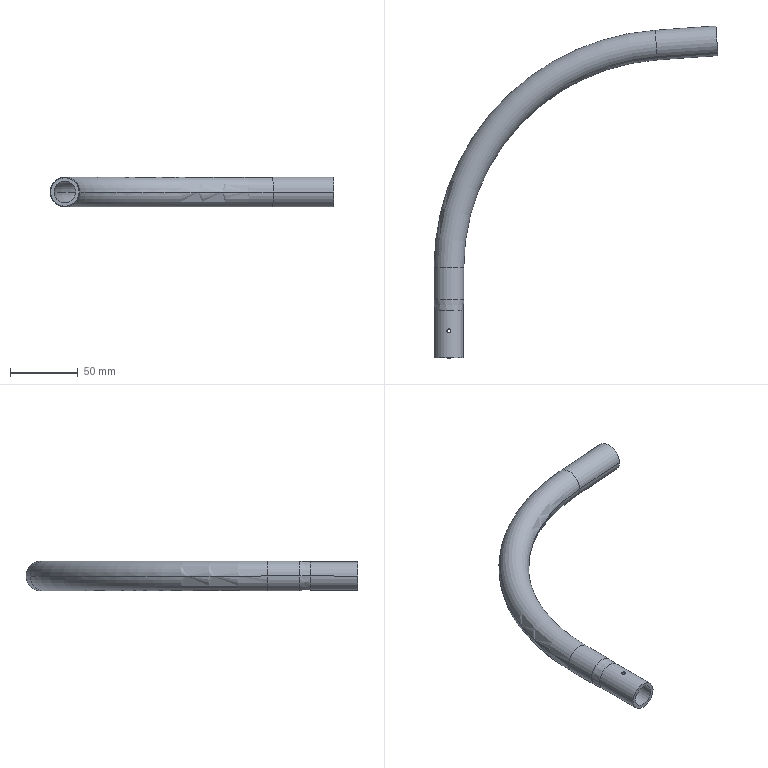Part | STEP file | 31E-01158WG10 | 1 solid | 22 faces | box 210.148 x 245.71 x 22 mm | volume 63051 mm3 | cylinder 14 | torus 4 | cone 2 | plane 2 | commonest cylinder face diameters 3 x4 16 x4 22 x4 21 x2
STEP:
#1=CARTESIAN_POINT('',(-1.316,20.719,-10.417));
#2=VERTEX_POINT('',#1);
#3=CARTESIAN_POINT('',(-1.316,20.719,-7.891));
#4=VERTEX_POINT('',#3);
#5=CARTESIAN_POINT('',(-1.316,20.719,-3.345));
#6=DIRECTION('',(0.,0.,-1.));
#7=VECTOR('',#6,1.);
#8=LINE('',#5,#7);
#9=EDGE_CURVE('',#2,#4,#8,.F.);
#10=ORIENTED_EDGE('',*,*,#9,.F.);
#11=CARTESIAN_POINT('',(1.316,19.281,-10.417));
#12=VERTEX_POINT('',#11);
#13=CARTESIAN_POINT('',(-1.316,20.719,-10.417));
#14=CARTESIAN_POINT('',(-1.132,21.056,-10.44));
#15=CARTESIAN_POINT('',(-0.8411,21.333,-10.473));
#16=CARTESIAN_POINT('',(-0.4667,21.506,-10.502));
#17=CARTESIAN_POINT('',(0.1367,21.567,-10.509));
#18=CARTESIAN_POINT('',(0.6816,21.357,-10.48));
#19=CARTESIAN_POINT('',(0.8505,21.258,-10.467));
#20=CARTESIAN_POINT('',(1.286,20.898,-10.426));
#21=CARTESIAN_POINT('',(1.526,20.366,-10.389));
#22=CARTESIAN_POINT('',(1.57,19.977,-10.381));
#23=CARTESIAN_POINT('',(1.492,19.602,-10.395));
#24=CARTESIAN_POINT('',(1.316,19.281,-10.417));
#25=B_SPLINE_CURVE_WITH_KNOTS('',5,(#13,#14,#15,#16,#17,#18,#19,#20,#21,#22,#23,#24),.UNSPECIFIED.,.F.,.U.,(6,3,3,6),(0.,2.718,4.081,6.673),.UNSPECIFIED.);
#26=EDGE_CURVE('',#2,#12,#25,.T.);
#27=ORIENTED_EDGE('',*,*,#26,.T.);
#28=CARTESIAN_POINT('',(1.316,19.281,-7.891));
#29=VERTEX_POINT('',#28);
#30=CARTESIAN_POINT('',(1.316,19.281,-3.345));
#31=DIRECTION('',(0.,0.,-1.));
#32=VECTOR('',#31,1.);
#33=LINE('',#30,#32);
#34=EDGE_CURVE('',#12,#29,#33,.F.);
#35=ORIENTED_EDGE('',*,*,#34,.T.);
#36=CARTESIAN_POINT('',(1.316,19.281,-7.891));
#37=CARTESIAN_POINT('',(1.5,19.618,-7.86));
#38=CARTESIAN_POINT('',(1.577,20.014,-7.842));
#39=CARTESIAN_POINT('',(1.518,20.425,-7.856));
#40=CARTESIAN_POINT('',(1.244,20.963,-7.911));
#41=CARTESIAN_POINT('',(0.7734,21.307,-7.965));
#42=CARTESIAN_POINT('',(0.5986,21.396,-7.981));
#43=CARTESIAN_POINT('',(0.05895,21.567,-8.012));
#44=CARTESIAN_POINT('',(-0.5205,21.481,-7.997));
#45=CARTESIAN_POINT('',(-0.8688,21.306,-7.961));
#46=CARTESIAN_POINT('',(-1.141,21.04,-7.92));
#47=CARTESIAN_POINT('',(-1.316,20.719,-7.891));
#48=B_SPLINE_CURVE_WITH_KNOTS('',5,(#36,#37,#38,#39,#40,#41,#42,#43,#44,#45,#46,#47),.UNSPECIFIED.,.F.,.U.,(6,3,3,6),(0.,2.721,4.087,6.679),.UNSPECIFIED.);
#49=EDGE_CURVE('',#29,#4,#48,.T.);
#50=ORIENTED_EDGE('',*,*,#49,.T.);
#51=EDGE_LOOP('',(#10,#27,#35,#50));
#52=FACE_OUTER_BOUND('',#51,.T.);
#53=CARTESIAN_POINT('',(0.,20.,-0.1));
#54=DIRECTION('',(0.,0.,-1.));
#55=DIRECTION('',(0.8776,-0.4794,0.));
#56=AXIS2_PLACEMENT_3D('',#53,#54,#55);
#57=CYLINDRICAL_SURFACE('',#56,1.5);
#58=ADVANCED_FACE('',(#52),#57,.F.);
#59=CARTESIAN_POINT('',(-8.,0.,0.));
#60=VERTEX_POINT('',#59);
#61=CARTESIAN_POINT('',(-8.,67.,0.));
#62=VERTEX_POINT('',#61);
#63=CARTESIAN_POINT('',(-8.,33.5,0.));
#64=DIRECTION('',(0.,1.,0.));
#65=VECTOR('',#64,1.);
#66=LINE('',#63,#65);
#67=EDGE_CURVE('',#60,#62,#66,.T.);
#68=ORIENTED_EDGE('',*,*,#67,.F.);
#69=CARTESIAN_POINT('',(8.,0.,0.));
#70=VERTEX_POINT('',#69);
#71=CARTESIAN_POINT('',(0.,0.,0.));
#72=DIRECTION('',(0.,1.,0.));
#73=AXIS2_PLACEMENT_3D('',#71,#72,$);
#74=CIRCLE('',#73,8.);
#75=EDGE_CURVE('',#70,#60,#74,.T.);
#76=ORIENTED_EDGE('',*,*,#75,.F.);
#77=CARTESIAN_POINT('',(8.,67.,0.));
#78=VERTEX_POINT('',#77);
#79=CARTESIAN_POINT('',(8.,33.5,0.));
#80=DIRECTION('',(0.,1.,0.));
#81=VECTOR('',#80,1.);
#82=LINE('',#79,#81);
#83=EDGE_CURVE('',#70,#78,#82,.T.);
#84=ORIENTED_EDGE('',*,*,#83,.T.);
#85=CARTESIAN_POINT('',(0.,67.,0.));
#86=DIRECTION('',(0.,1.,0.));
#87=AXIS2_PLACEMENT_3D('',#85,#86,$);
#88=CIRCLE('',#87,8.);
#89=EDGE_CURVE('',#62,#78,#88,.F.);
#90=ORIENTED_EDGE('',*,*,#89,.F.);
#91=EDGE_LOOP('',(#68,#76,#84,#90));
#92=FACE_OUTER_BOUND('',#91,.T.);
#93=ORIENTED_EDGE('',*,*,#49,.F.);
#94=CARTESIAN_POINT('',(1.316,19.281,-7.891));
#95=CARTESIAN_POINT('',(1.132,18.944,-7.922));
#96=CARTESIAN_POINT('',(0.8414,18.667,-7.965));
#97=CARTESIAN_POINT('',(0.4674,18.493,-8.002));
#98=CARTESIAN_POINT('',(-0.137,18.433,-8.012));
#99=CARTESIAN_POINT('',(-0.682,18.643,-7.974));
#100=CARTESIAN_POINT('',(-0.8508,18.742,-7.957));
#101=CARTESIAN_POINT('',(-1.285,19.102,-7.903));
#102=CARTESIAN_POINT('',(-1.526,19.633,-7.854));
#103=CARTESIAN_POINT('',(-1.57,20.023,-7.844));
#104=CARTESIAN_POINT('',(-1.492,20.398,-7.862));
#105=CARTESIAN_POINT('',(-1.316,20.719,-7.891));
#106=B_SPLINE_CURVE_WITH_KNOTS('',5,(#94,#95,#96,#97,#98,#99,#100,#101,#102,#103,#104,#105),.UNSPECIFIED.,.F.,.U.,(6,3,3,6),(0.,2.721,4.086,6.679),.UNSPECIFIED.);
#107=EDGE_CURVE('',#29,#4,#106,.T.);
#108=ORIENTED_EDGE('',*,*,#107,.T.);
#109=EDGE_LOOP('',(#93,#108));
#110=FACE_BOUND('',#109,.T.);
#111=CARTESIAN_POINT('',(0.,33.5,0.));
#112=DIRECTION('',(0.,1.,0.));
#113=DIRECTION('',(1.,0.,0.));
#114=AXIS2_PLACEMENT_3D('',#111,#112,#113);
#115=CYLINDRICAL_SURFACE('',#114,8.);
#116=ADVANCED_FACE('',(#92,#110),#115,.F.);
#117=CARTESIAN_POINT('',(1.316,19.281,-10.417));
#118=CARTESIAN_POINT('',(1.132,18.944,-10.44));
#119=CARTESIAN_POINT('',(0.8411,18.667,-10.473));
#120=CARTESIAN_POINT('',(0.4667,18.494,-10.502));
#121=CARTESIAN_POINT('',(-0.1367,18.433,-10.509));
#122=CARTESIAN_POINT('',(-0.6816,18.643,-10.48));
#123=CARTESIAN_POINT('',(-0.8505,18.742,-10.467));
#124=CARTESIAN_POINT('',(-1.286,19.102,-10.426));
#125=CARTESIAN_POINT('',(-1.526,19.634,-10.389));
#126=CARTESIAN_POINT('',(-1.57,20.023,-10.381));
#127=CARTESIAN_POINT('',(-1.492,20.398,-10.395));
#128=CARTESIAN_POINT('',(-1.316,20.719,-10.417));
#129=B_SPLINE_CURVE_WITH_KNOTS('',5,(#117,#118,#119,#120,#121,#122,#123,#124,#125,#126,#127,#128),.UNSPECIFIED.,.F.,.U.,(6,3,3,6),(0.,2.718,4.081,6.673),.UNSPECIFIED.);
#130=EDGE_CURVE('',#12,#2,#129,.T.);
#131=ORIENTED_EDGE('',*,*,#130,.T.);
#132=ORIENTED_EDGE('',*,*,#9,.T.);
#133=ORIENTED_EDGE('',*,*,#107,.F.);
#134=ORIENTED_EDGE('',*,*,#34,.F.);
#135=EDGE_LOOP('',(#131,#132,#133,#134));
#136=FACE_OUTER_BOUND('',#135,.T.);
#137=ADVANCED_FACE('',(#136),#57,.F.);
#138=CARTESIAN_POINT('',(-10.5,35.,0.));
#139=VERTEX_POINT('',#138);
#140=CARTESIAN_POINT('',(10.5,35.,0.));
#141=VERTEX_POINT('',#140);
#142=CARTESIAN_POINT('',(0.,35.,0.));
#143=DIRECTION('',(0.,-1.,0.));
#144=AXIS2_PLACEMENT_3D('',#142,#143,$);
#145=CIRCLE('',#144,10.5);
#146=EDGE_CURVE('',#139,#141,#145,.T.);
#147=ORIENTED_EDGE('',*,*,#146,.T.);
#148=CARTESIAN_POINT('',(10.5,0.,0.));
#149=VERTEX_POINT('',#148);
#150=CARTESIAN_POINT('',(10.5,17.5,0.));
#151=DIRECTION('',(0.,-1.,0.));
#152=VECTOR('',#151,1.);
#153=LINE('',#150,#152);
#154=EDGE_CURVE('',#149,#141,#153,.F.);
#155=ORIENTED_EDGE('',*,*,#154,.F.);
#156=CARTESIAN_POINT('',(-10.5,0.,0.));
#157=VERTEX_POINT('',#156);
#158=CARTESIAN_POINT('',(0.,0.,0.));
#159=DIRECTION('',(0.,-1.,0.));
#160=AXIS2_PLACEMENT_3D('',#158,#159,$);
#161=CIRCLE('',#160,10.5);
#162=EDGE_CURVE('',#157,#149,#161,.T.);
#163=ORIENTED_EDGE('',*,*,#162,.F.);
#164=CARTESIAN_POINT('',(-10.5,17.5,0.));
#165=DIRECTION('',(0.,-1.,0.));
#166=VECTOR('',#165,1.);
#167=LINE('',#164,#166);
#168=EDGE_CURVE('',#157,#139,#167,.F.);
#169=ORIENTED_EDGE('',*,*,#168,.T.);
#170=EDGE_LOOP('',(#147,#155,#163,#169));
#171=FACE_OUTER_BOUND('',#170,.T.);
#172=ORIENTED_EDGE('',*,*,#130,.F.);
#173=ORIENTED_EDGE('',*,*,#26,.F.);
#174=EDGE_LOOP('',(#172,#173));
#175=FACE_BOUND('',#174,.T.);
#176=CARTESIAN_POINT('',(0.,17.5,0.));
#177=DIRECTION('',(0.,-1.,0.));
#178=DIRECTION('',(1.,0.,0.));
#179=AXIS2_PLACEMENT_3D('',#176,#177,#178);
#180=CYLINDRICAL_SURFACE('',#179,10.5);
#181=ADVANCED_FACE('',(#171,#175),#180,.T.);
#182=ORIENTED_EDGE('',*,*,#83,.F.);
#183=CARTESIAN_POINT('',(0.,0.,0.));
#184=DIRECTION('',(0.,1.,0.));
#185=AXIS2_PLACEMENT_3D('',#183,#184,$);
#186=CIRCLE('',#185,8.);
#187=EDGE_CURVE('',#60,#70,#186,.T.);
#188=ORIENTED_EDGE('',*,*,#187,.F.);
#189=ORIENTED_EDGE('',*,*,#67,.T.);
#190=CARTESIAN_POINT('',(0.,67.,0.));
#191=DIRECTION('',(0.,1.,0.));
#192=AXIS2_PLACEMENT_3D('',#190,#191,$);
#193=CIRCLE('',#192,8.);
#194=EDGE_CURVE('',#78,#62,#193,.F.);
#195=ORIENTED_EDGE('',*,*,#194,.F.);
#196=EDGE_LOOP('',(#182,#188,#189,#195));
#197=FACE_OUTER_BOUND('',#196,.T.);
#198=CARTESIAN_POINT('',(1.316,20.719,7.891));
#199=VERTEX_POINT('',#198);
#200=CARTESIAN_POINT('',(-1.316,19.281,7.891));
#201=VERTEX_POINT('',#200);
#202=CARTESIAN_POINT('',(1.316,20.719,7.891));
#203=CARTESIAN_POINT('',(1.5,20.382,7.86));
#204=CARTESIAN_POINT('',(1.577,19.986,7.842));
#205=CARTESIAN_POINT('',(1.518,19.575,7.856));
#206=CARTESIAN_POINT('',(1.244,19.037,7.911));
#207=CARTESIAN_POINT('',(0.7734,18.693,7.965));
#208=CARTESIAN_POINT('',(0.5986,18.604,7.981));
#209=CARTESIAN_POINT('',(0.05895,18.433,8.012));
#210=CARTESIAN_POINT('',(-0.5205,18.519,7.997));
#211=CARTESIAN_POINT('',(-0.8688,18.694,7.961));
#212=CARTESIAN_POINT('',(-1.141,18.96,7.92));
#213=CARTESIAN_POINT('',(-1.316,19.281,7.891));
#214=B_SPLINE_CURVE_WITH_KNOTS('',5,(#202,#203,#204,#205,#206,#207,#208,#209,#210,#211,#212,#213),.UNSPECIFIED.,.F.,.U.,(6,3,3,6),(0.,2.721,4.087,6.679),.UNSPECIFIED.);
#215=EDGE_CURVE('',#199,#201,#214,.T.);
#216=ORIENTED_EDGE('',*,*,#215,.F.);
#217=CARTESIAN_POINT('',(-1.316,20.719,7.891));
#218=VERTEX_POINT('',#217);
#219=CARTESIAN_POINT('',(1.316,20.719,7.891));
#220=CARTESIAN_POINT('',(1.132,21.056,7.922));
#221=CARTESIAN_POINT('',(0.8414,21.333,7.965));
#222=CARTESIAN_POINT('',(0.4674,21.507,8.002));
#223=CARTESIAN_POINT('',(-0.2065,21.574,8.013));
#224=CARTESIAN_POINT('',(-0.8064,21.305,7.965));
#225=CARTESIAN_POINT('',(-1.02,21.146,7.938));
#226=CARTESIAN_POINT('',(-1.192,20.946,7.912));
#227=CARTESIAN_POINT('',(-1.316,20.719,7.891));
#228=B_SPLINE_CURVE_WITH_KNOTS('',5,(#219,#220,#221,#222,#223,#224,#225,#226,#227),.UNSPECIFIED.,.F.,.U.,(6,3,6),(0.,2.721,4.555),.UNSPECIFIED.);
#229=EDGE_CURVE('',#199,#218,#228,.T.);
#230=ORIENTED_EDGE('',*,*,#229,.T.);
#231=CARTESIAN_POINT('',(-1.316,20.719,7.891));
#232=CARTESIAN_POINT('',(-1.496,20.391,7.861));
#233=CARTESIAN_POINT('',(-1.567,20.,7.843));
#234=CARTESIAN_POINT('',(-1.496,19.609,7.861));
#235=CARTESIAN_POINT('',(-1.316,19.281,7.891));
#236=B_SPLINE_CURVE_WITH_KNOTS('',4,(#231,#232,#233,#234,#235),.UNSPECIFIED.,.F.,.U.,(5,5),(4.555,6.679),.UNSPECIFIED.);
#237=EDGE_CURVE('',#218,#201,#236,.T.);
#238=ORIENTED_EDGE('',*,*,#237,.T.);
#239=EDGE_LOOP('',(#216,#230,#238));
#240=FACE_BOUND('',#239,.T.);
#241=CARTESIAN_POINT('',(0.,33.5,0.));
#242=DIRECTION('',(0.,1.,0.));
#243=DIRECTION('',(-1.,0.,0.));
#244=AXIS2_PLACEMENT_3D('',#241,#242,#243);
#245=CYLINDRICAL_SURFACE('',#244,8.);
#246=ADVANCED_FACE('',(#197,#240),#245,.F.);
#247=CARTESIAN_POINT('',(0.,35.,0.));
#248=DIRECTION('',(0.,-1.,0.));
#249=AXIS2_PLACEMENT_3D('',#247,#248,$);
#250=CIRCLE('',#249,10.5);
#251=EDGE_CURVE('',#141,#139,#250,.T.);
#252=ORIENTED_EDGE('',*,*,#251,.T.);
#253=ORIENTED_EDGE('',*,*,#168,.F.);
#254=CARTESIAN_POINT('',(0.,0.,0.));
#255=DIRECTION('',(0.,-1.,0.));
#256=AXIS2_PLACEMENT_3D('',#254,#255,$);
#257=CIRCLE('',#256,10.5);
#258=EDGE_CURVE('',#149,#157,#257,.T.);
#259=ORIENTED_EDGE('',*,*,#258,.F.);
#260=ORIENTED_EDGE('',*,*,#154,.T.);
#261=EDGE_LOOP('',(#252,#253,#259,#260));
#262=FACE_OUTER_BOUND('',#261,.T.);
#263=CARTESIAN_POINT('',(-1.316,20.719,10.417));
#264=VERTEX_POINT('',#263);
#265=CARTESIAN_POINT('',(-1.316,19.281,10.417));
#266=VERTEX_POINT('',#265);
#267=CARTESIAN_POINT('',(-1.316,20.719,10.417));
#268=CARTESIAN_POINT('',(-1.496,20.39,10.394));
#269=CARTESIAN_POINT('',(-1.567,20.,10.381));
#270=CARTESIAN_POINT('',(-1.496,19.61,10.394));
#271=CARTESIAN_POINT('',(-1.316,19.281,10.417));
#272=B_SPLINE_CURVE_WITH_KNOTS('',4,(#267,#268,#269,#270,#271),.UNSPECIFIED.,.F.,.U.,(5,5),(4.55,6.673),.UNSPECIFIED.);
#273=EDGE_CURVE('',#264,#266,#272,.T.);
#274=ORIENTED_EDGE('',*,*,#273,.F.);
#275=CARTESIAN_POINT('',(1.316,20.719,10.417));
#276=VERTEX_POINT('',#275);
#277=CARTESIAN_POINT('',(1.316,20.719,10.417));
#278=CARTESIAN_POINT('',(1.008,21.283,10.456));
#279=CARTESIAN_POINT('',(0.4018,21.686,10.529));
#280=CARTESIAN_POINT('',(-0.4018,21.686,10.529));
#281=CARTESIAN_POINT('',(-1.008,21.283,10.456));
#282=CARTESIAN_POINT('',(-1.316,20.719,10.417));
#283=B_SPLINE_CURVE_WITH_KNOTS('',5,(#277,#278,#279,#280,#281,#282),.UNSPECIFIED.,.F.,.U.,(6,6),(0.,4.55),.UNSPECIFIED.);
#284=EDGE_CURVE('',#276,#264,#283,.T.);
#285=ORIENTED_EDGE('',*,*,#284,.F.);
#286=CARTESIAN_POINT('',(-1.316,19.281,10.417));
#287=CARTESIAN_POINT('',(-1.132,18.944,10.44));
#288=CARTESIAN_POINT('',(-0.8411,18.667,10.473));
#289=CARTESIAN_POINT('',(-0.4667,18.494,10.502));
#290=CARTESIAN_POINT('',(0.1367,18.433,10.509));
#291=CARTESIAN_POINT('',(0.6816,18.643,10.48));
#292=CARTESIAN_POINT('',(0.8505,18.742,10.467));
#293=CARTESIAN_POINT('',(1.286,19.102,10.426));
#294=CARTESIAN_POINT('',(1.526,19.634,10.389));
#295=CARTESIAN_POINT('',(1.57,20.023,10.381));
#296=CARTESIAN_POINT('',(1.492,20.398,10.395));
#297=CARTESIAN_POINT('',(1.316,20.719,10.417));
#298=B_SPLINE_CURVE_WITH_KNOTS('',5,(#286,#287,#288,#289,#290,#291,#292,#293,#294,#295,#296,#297),.UNSPECIFIED.,.F.,.U.,(6,3,3,6),(0.,2.718,4.081,6.673),.UNSPECIFIED.);
#299=EDGE_CURVE('',#266,#276,#298,.T.);
#300=ORIENTED_EDGE('',*,*,#299,.F.);
#301=EDGE_LOOP('',(#274,#285,#300));
#302=FACE_BOUND('',#301,.T.);
#303=ADVANCED_FACE('',(#262,#302),#180,.T.);
#304=CARTESIAN_POINT('',(-11.,43.,0.));
#305=VERTEX_POINT('',#304);
#306=CARTESIAN_POINT('',(-10.75,39.,0.));
#307=DIRECTION('',(-0.06238,0.9981,0.));
#308=VECTOR('',#307,1.);
#309=LINE('',#306,#308);
#310=EDGE_CURVE('',#139,#305,#309,.T.);
#311=ORIENTED_EDGE('',*,*,#310,.T.);
#312=CARTESIAN_POINT('',(11.,43.,0.));
#313=VERTEX_POINT('',#312);
#314=CARTESIAN_POINT('',(0.,43.,0.));
#315=DIRECTION('',(0.,-1.,0.));
#316=AXIS2_PLACEMENT_3D('',#314,#315,$);
#317=CIRCLE('',#316,11.);
#318=EDGE_CURVE('',#305,#313,#317,.T.);
#319=ORIENTED_EDGE('',*,*,#318,.T.);
#320=CARTESIAN_POINT('',(10.75,39.,0.));
#321=DIRECTION('',(0.06238,0.9981,0.));
#322=VECTOR('',#321,1.);
#323=LINE('',#320,#322);
#324=EDGE_CURVE('',#141,#313,#323,.T.);
#325=ORIENTED_EDGE('',*,*,#324,.F.);
#326=ORIENTED_EDGE('',*,*,#146,.F.);
#327=EDGE_LOOP('',(#311,#319,#325,#326));
#328=FACE_OUTER_BOUND('',#327,.T.);
#329=CARTESIAN_POINT('',(0.,-133.,0.));
#330=DIRECTION('',(0.,1.,0.));
#331=DIRECTION('',(-0.9072,0.,0.4207));
#332=AXIS2_PLACEMENT_3D('',#329,#330,#331);
#333=CONICAL_SURFACE('',#332,0.,0.06242);
#334=ADVANCED_FACE('',(#328),#333,.T.);
#335=CARTESIAN_POINT('',(-1.316,20.719,3.345));
#336=DIRECTION('',(0.,0.,1.));
#337=VECTOR('',#336,1.);
#338=LINE('',#335,#337);
#339=EDGE_CURVE('',#218,#264,#338,.T.);
#340=ORIENTED_EDGE('',*,*,#339,.F.);
#341=ORIENTED_EDGE('',*,*,#229,.F.);
#342=CARTESIAN_POINT('',(1.316,20.719,3.345));
#343=DIRECTION('',(0.,0.,1.));
#344=VECTOR('',#343,1.);
#345=LINE('',#342,#344);
#346=EDGE_CURVE('',#199,#276,#345,.T.);
#347=ORIENTED_EDGE('',*,*,#346,.T.);
#348=ORIENTED_EDGE('',*,*,#284,.T.);
#349=EDGE_LOOP('',(#340,#341,#347,#348));
#350=FACE_OUTER_BOUND('',#349,.T.);
#351=CARTESIAN_POINT('',(0.,20.,0.1));
#352=DIRECTION('',(0.,0.,1.));
#353=DIRECTION('',(0.8776,0.4794,0.));
#354=AXIS2_PLACEMENT_3D('',#351,#352,#353);
#355=CYLINDRICAL_SURFACE('',#354,1.5);
#356=ADVANCED_FACE('',(#350),#355,.F.);
#357=ORIENTED_EDGE('',*,*,#324,.T.);
#358=CARTESIAN_POINT('',(0.,43.,0.));
#359=DIRECTION('',(0.,-1.,0.));
#360=AXIS2_PLACEMENT_3D('',#358,#359,$);
#361=CIRCLE('',#360,11.);
#362=EDGE_CURVE('',#313,#305,#361,.T.);
#363=ORIENTED_EDGE('',*,*,#362,.T.);
#364=ORIENTED_EDGE('',*,*,#310,.F.);
#365=ORIENTED_EDGE('',*,*,#251,.F.);
#366=EDGE_LOOP('',(#357,#363,#364,#365));
#367=FACE_OUTER_BOUND('',#366,.T.);
#368=CARTESIAN_POINT('',(0.,-133.,0.));
#369=DIRECTION('',(0.,1.,0.));
#370=DIRECTION('',(0.9092,0.,-0.4163));
#371=AXIS2_PLACEMENT_3D('',#368,#369,#370);
#372=CONICAL_SURFACE('',#371,0.,0.06242);
#373=ADVANCED_FACE('',(#367),#372,.T.);
#374=CARTESIAN_POINT('',(-11.,67.,0.));
#375=VERTEX_POINT('',#374);
#376=CARTESIAN_POINT('',(-11.,33.5,0.));
#377=DIRECTION('',(0.,1.,0.));
#378=VECTOR('',#377,1.);
#379=LINE('',#376,#378);
#380=EDGE_CURVE('',#305,#375,#379,.T.);
#381=ORIENTED_EDGE('',*,*,#380,.T.);
#382=CARTESIAN_POINT('',(11.,67.,0.));
#383=VERTEX_POINT('',#382);
#384=CARTESIAN_POINT('',(0.,67.,0.));
#385=DIRECTION('',(0.,1.,0.));
#386=AXIS2_PLACEMENT_3D('',#384,#385,$);
#387=CIRCLE('',#386,11.);
#388=EDGE_CURVE('',#375,#383,#387,.F.);
#389=ORIENTED_EDGE('',*,*,#388,.T.);
#390=CARTESIAN_POINT('',(11.,33.5,0.));
#391=DIRECTION('',(0.,1.,0.));
#392=VECTOR('',#391,1.);
#393=LINE('',#390,#392);
#394=EDGE_CURVE('',#313,#383,#393,.T.);
#395=ORIENTED_EDGE('',*,*,#394,.F.);
#396=ORIENTED_EDGE('',*,*,#318,.F.);
#397=EDGE_LOOP('',(#381,#389,#395,#396));
#398=FACE_OUTER_BOUND('',#397,.T.);
#399=CARTESIAN_POINT('',(0.,33.5,0.));
#400=DIRECTION('',(0.,1.,0.));
#401=DIRECTION('',(1.,0.,0.));
#402=AXIS2_PLACEMENT_3D('',#399,#400,#401);
#403=CYLINDRICAL_SURFACE('',#402,11.);
#404=ADVANCED_FACE('',(#398),#403,.T.);
#405=ORIENTED_EDGE('',*,*,#394,.T.);
#406=CARTESIAN_POINT('',(0.,67.,0.));
#407=DIRECTION('',(0.,1.,0.));
#408=AXIS2_PLACEMENT_3D('',#406,#407,$);
#409=CIRCLE('',#408,11.);
#410=EDGE_CURVE('',#383,#375,#409,.F.);
#411=ORIENTED_EDGE('',*,*,#410,.T.);
#412=ORIENTED_EDGE('',*,*,#380,.F.);
#413=ORIENTED_EDGE('',*,*,#362,.F.);
#414=EDGE_LOOP('',(#405,#411,#412,#413));
#415=FACE_OUTER_BOUND('',#414,.T.);
#416=CARTESIAN_POINT('',(0.,33.5,0.));
#417=DIRECTION('',(0.,1.,0.));
#418=DIRECTION('',(-1.,0.,0.));
#419=AXIS2_PLACEMENT_3D('',#416,#417,#418);
#420=CYLINDRICAL_SURFACE('',#419,11.);
#421=ADVANCED_FACE('',(#415),#420,.T.);
#422=CARTESIAN_POINT('',(152.723,242.571,0.));
#423=VERTEX_POINT('',#422);
#424=CARTESIAN_POINT('',(165.,67.,0.));
#425=DIRECTION('',(0.,0.,1.));
#426=AXIS2_PLACEMENT_3D('',#424,#425,$);
#427=CIRCLE('',#426,176.);
#428=EDGE_CURVE('',#423,#375,#427,.T.);
#429=ORIENTED_EDGE('',*,*,#428,.F.);
#430=CARTESIAN_POINT('',(154.258,220.625,0.));
#431=VERTEX_POINT('',#430);
#432=CARTESIAN_POINT('',(153.49,231.598,0.));
#433=DIRECTION('',(0.9976,0.06976,0.));
#434=AXIS2_PLACEMENT_3D('',#432,#433,$);
#435=CIRCLE('',#434,11.);
#436=EDGE_CURVE('',#423,#431,#435,.F.);
#437=ORIENTED_EDGE('',*,*,#436,.T.);
#438=CARTESIAN_POINT('',(165.,67.,0.));
#439=DIRECTION('',(0.,0.,1.));
#440=AXIS2_PLACEMENT_3D('',#438,#439,$);
#441=CIRCLE('',#440,154.);
#442=EDGE_CURVE('',#431,#383,#441,.T.);
#443=ORIENTED_EDGE('',*,*,#442,.T.);
#444=ORIENTED_EDGE('',*,*,#388,.F.);
#445=EDGE_LOOP('',(#429,#437,#443,#444));
#446=FACE_OUTER_BOUND('',#445,.T.);
#447=CARTESIAN_POINT('',(165.,67.,0.));
#448=DIRECTION('',(0.,0.,1.));
#449=DIRECTION('',(-0.06976,0.9976,0.));
#450=AXIS2_PLACEMENT_3D('',#447,#448,#449);
#451=TOROIDAL_SURFACE('',#450,165.,11.);
#452=ADVANCED_FACE('',(#446),#451,.T.);
#453=ORIENTED_EDGE('',*,*,#442,.F.);
#454=CARTESIAN_POINT('',(153.49,231.598,0.));
#455=DIRECTION('',(0.9976,0.06976,0.));
#456=AXIS2_PLACEMENT_3D('',#454,#455,$);
#457=CIRCLE('',#456,11.);
#458=EDGE_CURVE('',#431,#423,#457,.F.);
#459=ORIENTED_EDGE('',*,*,#458,.T.);
#460=ORIENTED_EDGE('',*,*,#428,.T.);
#461=ORIENTED_EDGE('',*,*,#410,.F.);
#462=EDGE_LOOP('',(#453,#459,#460,#461));
#463=FACE_OUTER_BOUND('',#462,.T.);
#464=CARTESIAN_POINT('',(165.,67.,0.));
#465=DIRECTION('',(0.,0.,1.));
#466=DIRECTION('',(-0.06976,0.9976,0.));
#467=AXIS2_PLACEMENT_3D('',#464,#465,#466);
#468=TOROIDAL_SURFACE('',#467,165.,11.);
#469=ADVANCED_FACE('',(#463),#468,.T.);
#470=CARTESIAN_POINT('',(199.148,223.764,0.));
#471=VERTEX_POINT('',#470);
#472=CARTESIAN_POINT('',(197.613,245.71,0.));
#473=VERTEX_POINT('',#472);
#474=CARTESIAN_POINT('',(198.381,234.737,0.));
#475=DIRECTION('',(0.9976,0.06976,0.));
#476=AXIS2_PLACEMENT_3D('',#474,#475,$);
#477=CIRCLE('',#476,11.);
#478=EDGE_CURVE('',#471,#473,#477,.T.);
#479=ORIENTED_EDGE('',*,*,#478,.F.);
#480=CARTESIAN_POINT('',(176.703,222.194,0.));
#481=DIRECTION('',(0.9976,0.06976,0.));
#482=VECTOR('',#481,1.);
#483=LINE('',#480,#482);
#484=EDGE_CURVE('',#431,#471,#483,.T.);
#485=ORIENTED_EDGE('',*,*,#484,.F.);
#486=ORIENTED_EDGE('',*,*,#436,.F.);
#487=CARTESIAN_POINT('',(175.168,244.141,0.));
#488=DIRECTION('',(0.9976,0.06976,0.));
#489=VECTOR('',#488,1.);
#490=LINE('',#487,#489);
#491=EDGE_CURVE('',#423,#473,#490,.T.);
#492=ORIENTED_EDGE('',*,*,#491,.T.);
#493=EDGE_LOOP('',(#479,#485,#486,#492));
#494=FACE_OUTER_BOUND('',#493,.T.);
#495=CARTESIAN_POINT('',(175.935,233.168,0.));
#496=DIRECTION('',(0.9976,0.06976,0.));
#497=DIRECTION('',(0.06976,-0.9976,0.));
#498=AXIS2_PLACEMENT_3D('',#495,#496,#497);
#499=CYLINDRICAL_SURFACE('',#498,11.);
#500=ADVANCED_FACE('',(#494),#499,.T.);
#501=CARTESIAN_POINT('',(198.381,234.737,0.));
#502=DIRECTION('',(0.9976,0.06976,0.));
#503=AXIS2_PLACEMENT_3D('',#501,#502,$);
#504=CIRCLE('',#503,11.);
#505=EDGE_CURVE('',#473,#471,#504,.T.);
#506=ORIENTED_EDGE('',*,*,#505,.F.);
#507=ORIENTED_EDGE('',*,*,#491,.F.);
#508=ORIENTED_EDGE('',*,*,#458,.F.);
#509=ORIENTED_EDGE('',*,*,#484,.T.);
#510=EDGE_LOOP('',(#506,#507,#508,#509));
#511=FACE_OUTER_BOUND('',#510,.T.);
#512=CARTESIAN_POINT('',(175.935,233.168,0.));
#513=DIRECTION('',(0.9976,0.06976,0.));
#514=DIRECTION('',(-0.06976,0.9976,0.));
#515=AXIS2_PLACEMENT_3D('',#512,#513,#514);
#516=CYLINDRICAL_SURFACE('',#515,11.);
#517=ADVANCED_FACE('',(#511),#516,.T.);
#518=CARTESIAN_POINT('',(154.048,223.618,0.));
#519=VERTEX_POINT('',#518);
#520=CARTESIAN_POINT('',(198.939,226.757,0.));
#521=VERTEX_POINT('',#520);
#522=CARTESIAN_POINT('',(176.493,225.187,0.));
#523=DIRECTION('',(0.9976,0.06976,0.));
#524=VECTOR('',#523,1.);
#525=LINE('',#522,#524);
#526=EDGE_CURVE('',#519,#521,#525,.T.);
#527=ORIENTED_EDGE('',*,*,#526,.F.);
#528=CARTESIAN_POINT('',(152.932,239.579,0.));
#529=VERTEX_POINT('',#528);
#530=CARTESIAN_POINT('',(153.49,231.598,0.));
#531=DIRECTION('',(0.9976,0.06976,0.));
#532=AXIS2_PLACEMENT_3D('',#530,#531,$);
#533=CIRCLE('',#532,8.);
#534=EDGE_CURVE('',#519,#529,#533,.F.);
#535=ORIENTED_EDGE('',*,*,#534,.T.);
#536=CARTESIAN_POINT('',(197.823,242.718,0.));
#537=VERTEX_POINT('',#536);
#538=CARTESIAN_POINT('',(175.377,241.148,0.));
#539=DIRECTION('',(0.9976,0.06976,0.));
#540=VECTOR('',#539,1.);
#541=LINE('',#538,#540);
#542=EDGE_CURVE('',#529,#537,#541,.T.);
#543=ORIENTED_EDGE('',*,*,#542,.T.);
#544=CARTESIAN_POINT('',(198.381,234.737,0.));
#545=DIRECTION('',(0.9976,0.06976,0.));
#546=AXIS2_PLACEMENT_3D('',#544,#545,$);
#547=CIRCLE('',#546,8.);
#548=EDGE_CURVE('',#537,#521,#547,.T.);
#549=ORIENTED_EDGE('',*,*,#548,.T.);
#550=EDGE_LOOP('',(#527,#535,#543,#549));
#551=FACE_OUTER_BOUND('',#550,.T.);
#552=CARTESIAN_POINT('',(175.935,233.168,0.));
#553=DIRECTION('',(0.9976,0.06976,0.));
#554=DIRECTION('',(-0.06976,0.9976,0.));
#555=AXIS2_PLACEMENT_3D('',#552,#553,#554);
#556=CYLINDRICAL_SURFACE('',#555,8.);
#557=ADVANCED_FACE('',(#551),#556,.F.);
#558=ORIENTED_EDGE('',*,*,#542,.F.);
#559=CARTESIAN_POINT('',(153.49,231.598,0.));
#560=DIRECTION('',(0.9976,0.06976,0.));
#561=AXIS2_PLACEMENT_3D('',#559,#560,$);
#562=CIRCLE('',#561,8.);
#563=EDGE_CURVE('',#529,#519,#562,.F.);
#564=ORIENTED_EDGE('',*,*,#563,.T.);
#565=ORIENTED_EDGE('',*,*,#526,.T.);
#566=CARTESIAN_POINT('',(198.381,234.737,0.));
#567=DIRECTION('',(0.9976,0.06976,0.));
#568=AXIS2_PLACEMENT_3D('',#566,#567,$);
#569=CIRCLE('',#568,8.);
#570=EDGE_CURVE('',#521,#537,#569,.T.);
#571=ORIENTED_EDGE('',*,*,#570,.T.);
#572=EDGE_LOOP('',(#558,#564,#565,#571));
#573=FACE_OUTER_BOUND('',#572,.T.);
#574=CARTESIAN_POINT('',(175.935,233.168,0.));
#575=DIRECTION('',(0.9976,0.06976,0.));
#576=DIRECTION('',(0.06976,-0.9976,0.));
#577=AXIS2_PLACEMENT_3D('',#574,#575,#576);
#578=CYLINDRICAL_SURFACE('',#577,8.);
#579=ADVANCED_FACE('',(#573),#578,.F.);
#580=ORIENTED_EDGE('',*,*,#505,.T.);
#581=ORIENTED_EDGE('',*,*,#478,.T.);
#582=EDGE_LOOP('',(#580,#581));
#583=FACE_OUTER_BOUND('',#582,.T.);
#584=ORIENTED_EDGE('',*,*,#548,.F.);
#585=ORIENTED_EDGE('',*,*,#570,.F.);
#586=EDGE_LOOP('',(#584,#585));
#587=FACE_BOUND('',#586,.T.);
#588=CARTESIAN_POINT('',(198.381,234.737,0.));
#589=DIRECTION('',(0.9976,0.06976,0.));
#590=DIRECTION('',(-0.06976,0.9976,0.));
#591=AXIS2_PLACEMENT_3D('',#588,#589,#590);
#592=PLANE('',#591);
#593=ADVANCED_FACE('',(#583,#587),#592,.T.);
#594=ORIENTED_EDGE('',*,*,#194,.T.);
#595=CARTESIAN_POINT('',(165.,67.,0.));
#596=DIRECTION('',(0.,0.,1.));
#597=AXIS2_PLACEMENT_3D('',#595,#596,$);
#598=CIRCLE('',#597,173.);
#599=EDGE_CURVE('',#529,#62,#598,.T.);
#600=ORIENTED_EDGE('',*,*,#599,.F.);
#601=ORIENTED_EDGE('',*,*,#534,.F.);
#602=CARTESIAN_POINT('',(165.,67.,0.));
#603=DIRECTION('',(0.,0.,1.));
#604=AXIS2_PLACEMENT_3D('',#602,#603,$);
#605=CIRCLE('',#604,157.);
#606=EDGE_CURVE('',#519,#78,#605,.T.);
#607=ORIENTED_EDGE('',*,*,#606,.T.);
#608=EDGE_LOOP('',(#594,#600,#601,#607));
#609=FACE_OUTER_BOUND('',#608,.T.);
#610=CARTESIAN_POINT('',(165.,67.,0.));
#611=DIRECTION('',(0.,0.,1.));
#612=DIRECTION('',(-0.06976,0.9976,0.));
#613=AXIS2_PLACEMENT_3D('',#610,#611,#612);
#614=TOROIDAL_SURFACE('',#613,165.,8.);
#615=ADVANCED_FACE('',(#609),#614,.F.);
#616=ORIENTED_EDGE('',*,*,#162,.T.);
#617=ORIENTED_EDGE('',*,*,#258,.T.);
#618=EDGE_LOOP('',(#616,#617));
#619=FACE_OUTER_BOUND('',#618,.T.);
#620=ORIENTED_EDGE('',*,*,#187,.T.);
#621=ORIENTED_EDGE('',*,*,#75,.T.);
#622=EDGE_LOOP('',(#620,#621));
#623=FACE_BOUND('',#622,.T.);
#624=CARTESIAN_POINT('',(0.,0.,0.));
#625=DIRECTION('',(0.,1.,0.));
#626=DIRECTION('',(0.,0.,1.));
#627=AXIS2_PLACEMENT_3D('',#624,#625,#626);
#628=PLANE('',#627);
#629=ADVANCED_FACE('',(#619,#623),#628,.F.);
#630=ORIENTED_EDGE('',*,*,#89,.T.);
#631=ORIENTED_EDGE('',*,*,#606,.F.);
#632=ORIENTED_EDGE('',*,*,#563,.F.);
#633=ORIENTED_EDGE('',*,*,#599,.T.);
#634=EDGE_LOOP('',(#630,#631,#632,#633));
#635=FACE_OUTER_BOUND('',#634,.T.);
#636=CARTESIAN_POINT('',(165.,67.,0.));
#637=DIRECTION('',(0.,0.,1.));
#638=DIRECTION('',(-0.06976,0.9976,0.));
#639=AXIS2_PLACEMENT_3D('',#636,#637,#638);
#640=TOROIDAL_SURFACE('',#639,165.,8.);
#641=ADVANCED_FACE('',(#635),#640,.F.);
#642=ORIENTED_EDGE('',*,*,#339,.T.);
#643=ORIENTED_EDGE('',*,*,#273,.T.);
#644=ORIENTED_EDGE('',*,*,#299,.T.);
#645=ORIENTED_EDGE('',*,*,#346,.F.);
#646=ORIENTED_EDGE('',*,*,#215,.T.);
#647=ORIENTED_EDGE('',*,*,#237,.F.);
#648=EDGE_LOOP('',(#642,#643,#644,#645,#646,#647));
#649=FACE_OUTER_BOUND('',#648,.T.);
#650=ADVANCED_FACE('',(#649),#355,.F.);
#651=CLOSED_SHELL('',(#58,#116,#137,#181,#246,#303,#334,#356,#373,#404,#421,#452,#469,#500,#517,#557,#579,#593,#615,#629,#641,#650));
#652=MANIFOLD_SOLID_BREP('',#651);
#653=(LENGTH_UNIT()NAMED_UNIT(*)SI_UNIT(.MILLI.,.METRE.));
#654=UNCERTAINTY_MEASURE_WITH_UNIT(LENGTH_MEASURE(0.005),#653,'','');
#655=(NAMED_UNIT(*)PLANE_ANGLE_UNIT()SI_UNIT($,.RADIAN.));
#656=(NAMED_UNIT(*)SI_UNIT($,.STERADIAN.)SOLID_ANGLE_UNIT());
#657=(GEOMETRIC_REPRESENTATION_CONTEXT(3)GLOBAL_UNCERTAINTY_ASSIGNED_CONTEXT((#654))GLOBAL_UNIT_ASSIGNED_CONTEXT((#653,#655,#656))REPRESENTATION_CONTEXT('',''));
#658=ADVANCED_BREP_SHAPE_REPRESENTATION('',(#652),#657);